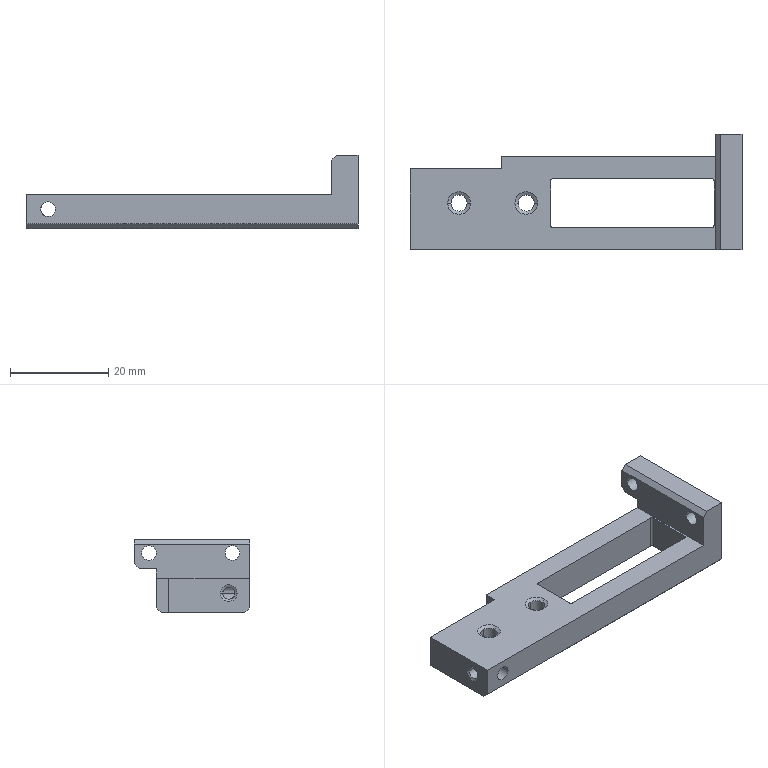Part | NX | 1 solid | 42 faces | box 67.7 x 23.5 x 15 mm | volume 6901 mm3 | plane 20 | cylinder 16 | cone 6 | commonest cylinder face diameters 3 x6 1 x4 3.3 x4 2.5 x2
STEP:
#1=CARTESIAN_POINT('',(-15.15,126.,-3.5));
#2=VERTEX_POINT('',#1);
#3=CARTESIAN_POINT('',(-33.85,126.,-3.5));
#4=VERTEX_POINT('',#3);
#5=CARTESIAN_POINT('',(0.,126.,-3.5));
#6=DIRECTION('',(-1.,0.,0.));
#7=VECTOR('',#6,1000.);
#8=LINE('',#5,#7);
#9=EDGE_CURVE('',#2,#4,#8,.T.);
#10=ORIENTED_EDGE('',*,*,#9,.T.);
#11=CARTESIAN_POINT('',(-33.85,126.,3.5));
#12=VERTEX_POINT('',#11);
#13=CARTESIAN_POINT('',(-33.85,126.,0.));
#14=DIRECTION('',(0.,0.,-1.));
#15=VECTOR('',#14,1000.);
#16=LINE('',#13,#15);
#17=EDGE_CURVE('',#12,#4,#16,.T.);
#18=ORIENTED_EDGE('',*,*,#17,.F.);
#19=CARTESIAN_POINT('',(-15.15,126.,3.5));
#20=VERTEX_POINT('',#19);
#21=CARTESIAN_POINT('',(0.,126.,3.5));
#22=DIRECTION('',(-1.,0.,0.));
#23=VECTOR('',#22,1000.);
#24=LINE('',#21,#23);
#25=EDGE_CURVE('',#20,#12,#24,.T.);
#26=ORIENTED_EDGE('',*,*,#25,.F.);
#27=CARTESIAN_POINT('',(-15.15,126.,-3.5));
#28=DIRECTION('',(0.,0.,1.));
#29=VECTOR('',#28,1000.);
#30=LINE('',#27,#29);
#31=EDGE_CURVE('',#2,#20,#30,.T.);
#32=ORIENTED_EDGE('',*,*,#31,.F.);
#33=EDGE_LOOP('',(#10,#18,#26,#32));
#34=FACE_BOUND('',#33,.T.);
#35=CARTESIAN_POINT('',(-30.85,126.,0.5));
#36=VERTEX_POINT('',#35);
#37=CARTESIAN_POINT('',(-27.85,126.,0.5));
#38=VERTEX_POINT('',#37);
#39=CARTESIAN_POINT('',(-29.35,126.,0.5));
#40=DIRECTION('',(0.,1.,0.));
#41=DIRECTION('',(-1.,0.,0.));
#42=AXIS2_PLACEMENT_3D('',#39,#40,#41);
#43=CIRCLE('',#42,1.5);
#44=EDGE_CURVE('',#36,#38,#43,.T.);
#45=ORIENTED_EDGE('',*,*,#44,.F.);
#46=CARTESIAN_POINT('',(-29.35,126.,0.5));
#47=DIRECTION('',(0.,1.,0.));
#48=DIRECTION('',(-1.,0.,0.));
#49=AXIS2_PLACEMENT_3D('',#46,#47,#48);
#50=CIRCLE('',#49,1.5);
#51=EDGE_CURVE('',#38,#36,#50,.T.);
#52=ORIENTED_EDGE('',*,*,#51,.F.);
#53=EDGE_LOOP('',(#45,#52));
#54=FACE_BOUND('',#53,.T.);
#55=CARTESIAN_POINT('',(-15.15,126.,3.5));
#56=DIRECTION('',(0.,1.,0.));
#57=DIRECTION('',(1.,0.,0.));
#58=AXIS2_PLACEMENT_3D('',#55,#56,#57);
#59=PLANE('',#58);
#60=ADVANCED_FACE('',(#34,#54),#59,.T.);
#61=CARTESIAN_POINT('',(-15.15,127.5,-3.5));
#62=VERTEX_POINT('',#61);
#63=CARTESIAN_POINT('',(-15.15,0.,-3.5));
#64=DIRECTION('',(0.,-1.,0.));
#65=VECTOR('',#64,1000.);
#66=LINE('',#63,#65);
#67=EDGE_CURVE('',#62,#2,#66,.T.);
#68=ORIENTED_EDGE('',*,*,#67,.T.);
#69=ORIENTED_EDGE('',*,*,#31,.T.);
#70=CARTESIAN_POINT('',(-15.15,128.5,3.5));
#71=VERTEX_POINT('',#70);
#72=CARTESIAN_POINT('',(-15.15,0.,3.5));
#73=DIRECTION('',(0.,-1.,0.));
#74=VECTOR('',#73,1000.);
#75=LINE('',#72,#74);
#76=EDGE_CURVE('',#71,#20,#75,.T.);
#77=ORIENTED_EDGE('',*,*,#76,.F.);
#78=CARTESIAN_POINT('',(-15.15,128.5,-2.5));
#79=VERTEX_POINT('',#78);
#80=CARTESIAN_POINT('',(-15.15,128.5,0.));
#81=DIRECTION('',(0.,0.,1.));
#82=VECTOR('',#81,1000.);
#83=LINE('',#80,#82);
#84=EDGE_CURVE('',#79,#71,#83,.T.);
#85=ORIENTED_EDGE('',*,*,#84,.F.);
#86=CARTESIAN_POINT('',(-15.15,127.5,-3.5));
#87=DIRECTION('',(0.,0.7071,0.7071));
#88=VECTOR('',#87,1000.);
#89=LINE('',#86,#88);
#90=EDGE_CURVE('',#62,#79,#89,.T.);
#91=ORIENTED_EDGE('',*,*,#90,.F.);
#92=EDGE_LOOP('',(#68,#69,#77,#85,#91));
#93=FACE_BOUND('',#92,.T.);
#94=CARTESIAN_POINT('',(-15.15,128.5,3.5));
#95=DIRECTION('',(-1.,0.,0.));
#96=DIRECTION('',(0.,0.,1.));
#97=AXIS2_PLACEMENT_3D('',#94,#95,#96);
#98=PLANE('',#97);
#99=ADVANCED_FACE('',(#93),#98,.T.);
#100=CARTESIAN_POINT('',(33.85,127.5,-3.5));
#101=VERTEX_POINT('',#100);
#102=CARTESIAN_POINT('',(0.,127.5,-3.5));
#103=DIRECTION('',(1.,0.,0.));
#104=VECTOR('',#103,1000.);
#105=LINE('',#102,#104);
#106=EDGE_CURVE('',#62,#101,#105,.T.);
#107=ORIENTED_EDGE('',*,*,#106,.F.);
#108=ORIENTED_EDGE('',*,*,#90,.T.);
#109=CARTESIAN_POINT('',(33.85,128.5,-2.5));
#110=VERTEX_POINT('',#109);
#111=CARTESIAN_POINT('',(0.,128.5,-2.5));
#112=DIRECTION('',(1.,0.,0.));
#113=VECTOR('',#112,1000.);
#114=LINE('',#111,#113);
#115=EDGE_CURVE('',#79,#110,#114,.T.);
#116=ORIENTED_EDGE('',*,*,#115,.T.);
#117=CARTESIAN_POINT('',(33.85,131.,0.));
#118=DIRECTION('',(0.,-0.7071,-0.7071));
#119=VECTOR('',#118,1000.);
#120=LINE('',#117,#119);
#121=EDGE_CURVE('',#110,#101,#120,.T.);
#122=ORIENTED_EDGE('',*,*,#121,.T.);
#123=EDGE_LOOP('',(#107,#108,#116,#122));
#124=FACE_BOUND('',#123,.T.);
#125=CARTESIAN_POINT('',(-15.15,127.5,-3.5));
#126=DIRECTION('',(0.,-0.7071,0.7071));
#127=DIRECTION('',(-1.,0.,0.));
#128=AXIS2_PLACEMENT_3D('',#125,#126,#127);
#129=PLANE('',#128);
#130=ADVANCED_FACE('',(#124),#129,.F.);
#131=ORIENTED_EDGE('',*,*,#76,.T.);
#132=ORIENTED_EDGE('',*,*,#25,.T.);
#133=CARTESIAN_POINT('',(-33.85,109.5,3.5));
#134=VERTEX_POINT('',#133);
#135=CARTESIAN_POINT('',(-33.85,0.,3.5));
#136=DIRECTION('',(0.,-1.,0.));
#137=VECTOR('',#136,1000.);
#138=LINE('',#135,#137);
#139=EDGE_CURVE('',#12,#134,#138,.T.);
#140=ORIENTED_EDGE('',*,*,#139,.T.);
#141=CARTESIAN_POINT('',(28.5,109.5,3.5));
#142=VERTEX_POINT('',#141);
#143=CARTESIAN_POINT('',(0.,109.5,3.5));
#144=DIRECTION('',(-1.,0.,0.));
#145=VECTOR('',#144,1000.);
#146=LINE('',#143,#145);
#147=EDGE_CURVE('',#142,#134,#146,.T.);
#148=ORIENTED_EDGE('',*,*,#147,.F.);
#149=CARTESIAN_POINT('',(28.5,128.5,3.5));
#150=VERTEX_POINT('',#149);
#151=CARTESIAN_POINT('',(28.5,0.,3.5));
#152=DIRECTION('',(0.,1.,0.));
#153=VECTOR('',#152,1000.);
#154=LINE('',#151,#153);
#155=EDGE_CURVE('',#142,#150,#154,.T.);
#156=ORIENTED_EDGE('',*,*,#155,.T.);
#157=CARTESIAN_POINT('',(0.,128.5,3.5));
#158=DIRECTION('',(1.,0.,0.));
#159=VECTOR('',#158,1000.);
#160=LINE('',#157,#159);
#161=EDGE_CURVE('',#71,#150,#160,.T.);
#162=ORIENTED_EDGE('',*,*,#161,.F.);
#163=EDGE_LOOP('',(#131,#132,#140,#148,#156,#162));
#164=FACE_BOUND('',#163,.T.);
#165=CARTESIAN_POINT('',(-4.65,124.,3.5));
#166=VERTEX_POINT('',#165);
#167=CARTESIAN_POINT('',(27.65,124.,3.5));
#168=VERTEX_POINT('',#167);
#169=CARTESIAN_POINT('',(0.,124.,3.5));
#170=DIRECTION('',(1.,0.,0.));
#171=VECTOR('',#170,1000.);
#172=LINE('',#169,#171);
#173=EDGE_CURVE('',#166,#168,#172,.T.);
#174=ORIENTED_EDGE('',*,*,#173,.T.);
#175=CARTESIAN_POINT('',(28.15,123.5,3.5));
#176=VERTEX_POINT('',#175);
#177=CARTESIAN_POINT('',(27.65,123.5,3.5));
#178=DIRECTION('',(0.,0.,-1.));
#179=DIRECTION('',(0.,-1.,0.));
#180=AXIS2_PLACEMENT_3D('',#177,#178,#179);
#181=CIRCLE('',#180,0.5);
#182=EDGE_CURVE('',#168,#176,#181,.T.);
#183=ORIENTED_EDGE('',*,*,#182,.T.);
#184=CARTESIAN_POINT('',(28.15,114.5,3.5));
#185=VERTEX_POINT('',#184);
#186=CARTESIAN_POINT('',(28.15,0.,3.5));
#187=DIRECTION('',(0.,-1.,0.));
#188=VECTOR('',#187,1000.);
#189=LINE('',#186,#188);
#190=EDGE_CURVE('',#176,#185,#189,.T.);
#191=ORIENTED_EDGE('',*,*,#190,.T.);
#192=CARTESIAN_POINT('',(27.65,114.,3.5));
#193=VERTEX_POINT('',#192);
#194=CARTESIAN_POINT('',(27.65,114.5,3.5));
#195=DIRECTION('',(0.,0.,-1.));
#196=DIRECTION('',(0.,-1.,0.));
#197=AXIS2_PLACEMENT_3D('',#194,#195,#196);
#198=CIRCLE('',#197,0.5);
#199=EDGE_CURVE('',#185,#193,#198,.T.);
#200=ORIENTED_EDGE('',*,*,#199,.T.);
#201=CARTESIAN_POINT('',(-4.65,114.,3.5));
#202=VERTEX_POINT('',#201);
#203=CARTESIAN_POINT('',(0.,114.,3.5));
#204=DIRECTION('',(-1.,0.,0.));
#205=VECTOR('',#204,1000.);
#206=LINE('',#203,#205);
#207=EDGE_CURVE('',#193,#202,#206,.T.);
#208=ORIENTED_EDGE('',*,*,#207,.T.);
#209=CARTESIAN_POINT('',(-5.15,114.5,3.5));
#210=VERTEX_POINT('',#209);
#211=CARTESIAN_POINT('',(-4.65,114.5,3.5));
#212=DIRECTION('',(0.,0.,-1.));
#213=DIRECTION('',(0.,-1.,0.));
#214=AXIS2_PLACEMENT_3D('',#211,#212,#213);
#215=CIRCLE('',#214,0.5);
#216=EDGE_CURVE('',#202,#210,#215,.T.);
#217=ORIENTED_EDGE('',*,*,#216,.T.);
#218=CARTESIAN_POINT('',(-5.15,123.5,3.5));
#219=VERTEX_POINT('',#218);
#220=CARTESIAN_POINT('',(-5.15,0.,3.5));
#221=DIRECTION('',(0.,1.,0.));
#222=VECTOR('',#221,1000.);
#223=LINE('',#220,#222);
#224=EDGE_CURVE('',#210,#219,#223,.T.);
#225=ORIENTED_EDGE('',*,*,#224,.T.);
#226=CARTESIAN_POINT('',(-4.65,123.5,3.5));
#227=DIRECTION('',(0.,0.,-1.));
#228=DIRECTION('',(0.,-1.,0.));
#229=AXIS2_PLACEMENT_3D('',#226,#227,#228);
#230=CIRCLE('',#229,0.5);
#231=EDGE_CURVE('',#219,#166,#230,.T.);
#232=ORIENTED_EDGE('',*,*,#231,.T.);
#233=EDGE_LOOP('',(#174,#183,#191,#200,#208,#217,#225,#232));
#234=FACE_BOUND('',#233,.T.);
#235=CARTESIAN_POINT('',(-21.535,119.,3.5));
#236=VERTEX_POINT('',#235);
#237=CARTESIAN_POINT('',(-26.165,119.,3.5));
#238=VERTEX_POINT('',#237);
#239=CARTESIAN_POINT('',(-23.85,119.,3.5));
#240=DIRECTION('',(0.,0.,1.));
#241=DIRECTION('',(1.,0.,0.));
#242=AXIS2_PLACEMENT_3D('',#239,#240,#241);
#243=CIRCLE('',#242,2.315);
#244=EDGE_CURVE('',#236,#238,#243,.T.);
#245=ORIENTED_EDGE('',*,*,#244,.F.);
#246=CARTESIAN_POINT('',(-23.85,119.,3.5));
#247=DIRECTION('',(0.,0.,1.));
#248=DIRECTION('',(1.,0.,0.));
#249=AXIS2_PLACEMENT_3D('',#246,#247,#248);
#250=CIRCLE('',#249,2.315);
#251=EDGE_CURVE('',#238,#236,#250,.T.);
#252=ORIENTED_EDGE('',*,*,#251,.F.);
#253=EDGE_LOOP('',(#245,#252));
#254=FACE_BOUND('',#253,.T.);
#255=CARTESIAN_POINT('',(-12.465,119.,3.5));
#256=VERTEX_POINT('',#255);
#257=CARTESIAN_POINT('',(-7.835,119.,3.5));
#258=VERTEX_POINT('',#257);
#259=CARTESIAN_POINT('',(-10.15,119.,3.5));
#260=DIRECTION('',(0.,0.,1.));
#261=DIRECTION('',(1.,0.,0.));
#262=AXIS2_PLACEMENT_3D('',#259,#260,#261);
#263=CIRCLE('',#262,2.315);
#264=EDGE_CURVE('',#256,#258,#263,.T.);
#265=ORIENTED_EDGE('',*,*,#264,.F.);
#266=CARTESIAN_POINT('',(-10.15,119.,3.5));
#267=DIRECTION('',(0.,0.,1.));
#268=DIRECTION('',(1.,0.,0.));
#269=AXIS2_PLACEMENT_3D('',#266,#267,#268);
#270=CIRCLE('',#269,2.315);
#271=EDGE_CURVE('',#258,#256,#270,.T.);
#272=ORIENTED_EDGE('',*,*,#271,.F.);
#273=EDGE_LOOP('',(#265,#272));
#274=FACE_BOUND('',#273,.T.);
#275=CARTESIAN_POINT('',(0.,119.,3.5));
#276=DIRECTION('',(0.,0.,-1.));
#277=DIRECTION('',(0.,-1.,0.));
#278=AXIS2_PLACEMENT_3D('',#275,#276,#277);
#279=PLANE('',#278);
#280=ADVANCED_FACE('',(#164,#234,#254,#274),#279,.F.);
#281=CARTESIAN_POINT('',(29.5,109.5,11.5));
#282=VERTEX_POINT('',#281);
#283=CARTESIAN_POINT('',(29.5,133.,11.5));
#284=VERTEX_POINT('',#283);
#285=CARTESIAN_POINT('',(29.5,0.,11.5));
#286=DIRECTION('',(0.,1.,0.));
#287=VECTOR('',#286,1000.);
#288=LINE('',#285,#287);
#289=EDGE_CURVE('',#282,#284,#288,.T.);
#290=ORIENTED_EDGE('',*,*,#289,.F.);
#291=CARTESIAN_POINT('',(33.85,109.5,11.5));
#292=VERTEX_POINT('',#291);
#293=CARTESIAN_POINT('',(0.,109.5,11.5));
#294=DIRECTION('',(1.,0.,0.));
#295=VECTOR('',#294,1000.);
#296=LINE('',#293,#295);
#297=EDGE_CURVE('',#282,#292,#296,.T.);
#298=ORIENTED_EDGE('',*,*,#297,.T.);
#299=CARTESIAN_POINT('',(33.85,133.,11.5));
#300=VERTEX_POINT('',#299);
#301=CARTESIAN_POINT('',(33.85,0.,11.5));
#302=DIRECTION('',(0.,1.,0.));
#303=VECTOR('',#302,1000.);
#304=LINE('',#301,#303);
#305=EDGE_CURVE('',#292,#300,#304,.T.);
#306=ORIENTED_EDGE('',*,*,#305,.T.);
#307=CARTESIAN_POINT('',(0.,133.,11.5));
#308=DIRECTION('',(1.,0.,0.));
#309=VECTOR('',#308,1000.);
#310=LINE('',#307,#309);
#311=EDGE_CURVE('',#284,#300,#310,.T.);
#312=ORIENTED_EDGE('',*,*,#311,.F.);
#313=EDGE_LOOP('',(#290,#298,#306,#312));
#314=FACE_BOUND('',#313,.T.);
#315=CARTESIAN_POINT('',(0.,119.,11.5));
#316=DIRECTION('',(0.,0.,-1.));
#317=DIRECTION('',(0.,-1.,0.));
#318=AXIS2_PLACEMENT_3D('',#315,#316,#317);
#319=PLANE('',#318);
#320=ADVANCED_FACE('',(#314),#319,.F.);
#321=CARTESIAN_POINT('',(28.5,109.5,10.5));
#322=VERTEX_POINT('',#321);
#323=CARTESIAN_POINT('',(28.5,133.,10.5));
#324=VERTEX_POINT('',#323);
#325=CARTESIAN_POINT('',(28.5,0.,10.5));
#326=DIRECTION('',(0.,1.,0.));
#327=VECTOR('',#326,1000.);
#328=LINE('',#325,#327);
#329=EDGE_CURVE('',#322,#324,#328,.T.);
#330=ORIENTED_EDGE('',*,*,#329,.F.);
#331=CARTESIAN_POINT('',(18.,109.5,0.));
#332=DIRECTION('',(-0.7071,0.,-0.7071));
#333=VECTOR('',#332,1000.);
#334=LINE('',#331,#333);
#335=EDGE_CURVE('',#282,#322,#334,.T.);
#336=ORIENTED_EDGE('',*,*,#335,.F.);
#337=ORIENTED_EDGE('',*,*,#289,.T.);
#338=CARTESIAN_POINT('',(18.,133.,0.));
#339=DIRECTION('',(-0.7071,0.,-0.7071));
#340=VECTOR('',#339,1000.);
#341=LINE('',#338,#340);
#342=EDGE_CURVE('',#284,#324,#341,.T.);
#343=ORIENTED_EDGE('',*,*,#342,.T.);
#344=EDGE_LOOP('',(#330,#336,#337,#343));
#345=FACE_BOUND('',#344,.T.);
#346=CARTESIAN_POINT('',(28.5,129.5,10.5));
#347=DIRECTION('',(-0.7071,0.,0.7071));
#348=DIRECTION('',(0.,1.,0.));
#349=AXIS2_PLACEMENT_3D('',#346,#347,#348);
#350=PLANE('',#349);
#351=ADVANCED_FACE('',(#345),#350,.T.);
#352=CARTESIAN_POINT('',(-33.85,110.5,-3.5));
#353=VERTEX_POINT('',#352);
#354=CARTESIAN_POINT('',(33.85,110.5,-3.5));
#355=VERTEX_POINT('',#354);
#356=CARTESIAN_POINT('',(0.,110.5,-3.5));
#357=DIRECTION('',(1.,0.,0.));
#358=VECTOR('',#357,1000.);
#359=LINE('',#356,#358);
#360=EDGE_CURVE('',#353,#355,#359,.T.);
#361=ORIENTED_EDGE('',*,*,#360,.F.);
#362=CARTESIAN_POINT('',(-33.85,0.,-3.5));
#363=DIRECTION('',(0.,-1.,0.));
#364=VECTOR('',#363,1000.);
#365=LINE('',#362,#364);
#366=EDGE_CURVE('',#4,#353,#365,.T.);
#367=ORIENTED_EDGE('',*,*,#366,.F.);
#368=ORIENTED_EDGE('',*,*,#9,.F.);
#369=ORIENTED_EDGE('',*,*,#67,.F.);
#370=ORIENTED_EDGE('',*,*,#106,.T.);
#371=CARTESIAN_POINT('',(33.85,0.,-3.5));
#372=DIRECTION('',(0.,-1.,0.));
#373=VECTOR('',#372,1000.);
#374=LINE('',#371,#373);
#375=EDGE_CURVE('',#101,#355,#374,.T.);
#376=ORIENTED_EDGE('',*,*,#375,.T.);
#377=EDGE_LOOP('',(#361,#367,#368,#369,#370,#376));
#378=FACE_BOUND('',#377,.T.);
#379=CARTESIAN_POINT('',(-4.65,124.,-3.5));
#380=VERTEX_POINT('',#379);
#381=CARTESIAN_POINT('',(27.65,124.,-3.5));
#382=VERTEX_POINT('',#381);
#383=CARTESIAN_POINT('',(0.,124.,-3.5));
#384=DIRECTION('',(1.,0.,0.));
#385=VECTOR('',#384,1000.);
#386=LINE('',#383,#385);
#387=EDGE_CURVE('',#380,#382,#386,.T.);
#388=ORIENTED_EDGE('',*,*,#387,.F.);
#389=CARTESIAN_POINT('',(-5.15,123.5,-3.5));
#390=VERTEX_POINT('',#389);
#391=CARTESIAN_POINT('',(-4.65,123.5,-3.5));
#392=DIRECTION('',(0.,0.,-1.));
#393=DIRECTION('',(0.,-1.,0.));
#394=AXIS2_PLACEMENT_3D('',#391,#392,#393);
#395=CIRCLE('',#394,0.5);
#396=EDGE_CURVE('',#390,#380,#395,.T.);
#397=ORIENTED_EDGE('',*,*,#396,.F.);
#398=CARTESIAN_POINT('',(-5.15,114.5,-3.5));
#399=VERTEX_POINT('',#398);
#400=CARTESIAN_POINT('',(-5.15,0.,-3.5));
#401=DIRECTION('',(0.,1.,0.));
#402=VECTOR('',#401,1000.);
#403=LINE('',#400,#402);
#404=EDGE_CURVE('',#399,#390,#403,.T.);
#405=ORIENTED_EDGE('',*,*,#404,.F.);
#406=CARTESIAN_POINT('',(-4.65,114.,-3.5));
#407=VERTEX_POINT('',#406);
#408=CARTESIAN_POINT('',(-4.65,114.5,-3.5));
#409=DIRECTION('',(0.,0.,-1.));
#410=DIRECTION('',(0.,-1.,0.));
#411=AXIS2_PLACEMENT_3D('',#408,#409,#410);
#412=CIRCLE('',#411,0.5);
#413=EDGE_CURVE('',#407,#399,#412,.T.);
#414=ORIENTED_EDGE('',*,*,#413,.F.);
#415=CARTESIAN_POINT('',(27.65,114.,-3.5));
#416=VERTEX_POINT('',#415);
#417=CARTESIAN_POINT('',(0.,114.,-3.5));
#418=DIRECTION('',(-1.,0.,0.));
#419=VECTOR('',#418,1000.);
#420=LINE('',#417,#419);
#421=EDGE_CURVE('',#416,#407,#420,.T.);
#422=ORIENTED_EDGE('',*,*,#421,.F.);
#423=CARTESIAN_POINT('',(28.15,114.5,-3.5));
#424=VERTEX_POINT('',#423);
#425=CARTESIAN_POINT('',(27.65,114.5,-3.5));
#426=DIRECTION('',(0.,0.,-1.));
#427=DIRECTION('',(0.,-1.,0.));
#428=AXIS2_PLACEMENT_3D('',#425,#426,#427);
#429=CIRCLE('',#428,0.5);
#430=EDGE_CURVE('',#424,#416,#429,.T.);
#431=ORIENTED_EDGE('',*,*,#430,.F.);
#432=CARTESIAN_POINT('',(28.15,123.5,-3.5));
#433=VERTEX_POINT('',#432);
#434=CARTESIAN_POINT('',(28.15,0.,-3.5));
#435=DIRECTION('',(0.,-1.,0.));
#436=VECTOR('',#435,1000.);
#437=LINE('',#434,#436);
#438=EDGE_CURVE('',#433,#424,#437,.T.);
#439=ORIENTED_EDGE('',*,*,#438,.F.);
#440=CARTESIAN_POINT('',(27.65,123.5,-3.5));
#441=DIRECTION('',(0.,0.,-1.));
#442=DIRECTION('',(0.,-1.,0.));
#443=AXIS2_PLACEMENT_3D('',#440,#441,#442);
#444=CIRCLE('',#443,0.5);
#445=EDGE_CURVE('',#382,#433,#444,.T.);
#446=ORIENTED_EDGE('',*,*,#445,.F.);
#447=EDGE_LOOP('',(#388,#397,#405,#414,#422,#431,#439,#446));
#448=FACE_BOUND('',#447,.T.);
#449=CARTESIAN_POINT('',(-10.15,117.35,-3.5));
#450=VERTEX_POINT('',#449);
#451=CARTESIAN_POINT('',(-10.15,120.65,-3.5));
#452=VERTEX_POINT('',#451);
#453=CARTESIAN_POINT('',(-10.15,119.,-3.5));
#454=DIRECTION('',(0.,0.,1.));
#455=DIRECTION('',(0.,1.,0.));
#456=AXIS2_PLACEMENT_3D('',#453,#454,#455);
#457=CIRCLE('',#456,1.65);
#458=EDGE_CURVE('',#450,#452,#457,.T.);
#459=ORIENTED_EDGE('',*,*,#458,.T.);
#460=CARTESIAN_POINT('',(-10.15,119.,-3.5));
#461=DIRECTION('',(0.,0.,1.));
#462=DIRECTION('',(0.,1.,0.));
#463=AXIS2_PLACEMENT_3D('',#460,#461,#462);
#464=CIRCLE('',#463,1.65);
#465=EDGE_CURVE('',#452,#450,#464,.T.);
#466=ORIENTED_EDGE('',*,*,#465,.T.);
#467=EDGE_LOOP('',(#459,#466));
#468=FACE_BOUND('',#467,.T.);
#469=CARTESIAN_POINT('',(-23.85,117.35,-3.5));
#470=VERTEX_POINT('',#469);
#471=CARTESIAN_POINT('',(-23.85,120.65,-3.5));
#472=VERTEX_POINT('',#471);
#473=CARTESIAN_POINT('',(-23.85,119.,-3.5));
#474=DIRECTION('',(0.,0.,1.));
#475=DIRECTION('',(0.,1.,0.));
#476=AXIS2_PLACEMENT_3D('',#473,#474,#475);
#477=CIRCLE('',#476,1.65);
#478=EDGE_CURVE('',#470,#472,#477,.T.);
#479=ORIENTED_EDGE('',*,*,#478,.T.);
#480=CARTESIAN_POINT('',(-23.85,119.,-3.5));
#481=DIRECTION('',(0.,0.,1.));
#482=DIRECTION('',(0.,1.,0.));
#483=AXIS2_PLACEMENT_3D('',#480,#481,#482);
#484=CIRCLE('',#483,1.65);
#485=EDGE_CURVE('',#472,#470,#484,.T.);
#486=ORIENTED_EDGE('',*,*,#485,.T.);
#487=EDGE_LOOP('',(#479,#486));
#488=FACE_BOUND('',#487,.T.);
#489=CARTESIAN_POINT('',(0.,119.,-3.5));
#490=DIRECTION('',(0.,0.,-1.));
#491=DIRECTION('',(0.,-1.,0.));
#492=AXIS2_PLACEMENT_3D('',#489,#490,#491);
#493=PLANE('',#492);
#494=ADVANCED_FACE('',(#378,#448,#468,#488),#493,.T.);
#495=CARTESIAN_POINT('',(28.5,128.5,5.5));
#496=VERTEX_POINT('',#495);
#497=CARTESIAN_POINT('',(33.85,128.5,5.5));
#498=VERTEX_POINT('',#497);
#499=CARTESIAN_POINT('',(0.,128.5,5.5));
#500=DIRECTION('',(1.,0.,0.));
#501=VECTOR('',#500,1000.);
#502=LINE('',#499,#501);
#503=EDGE_CURVE('',#496,#498,#502,.T.);
#504=ORIENTED_EDGE('',*,*,#503,.T.);
#505=CARTESIAN_POINT('',(33.85,128.5,0.));
#506=DIRECTION('',(0.,0.,-1.));
#507=VECTOR('',#506,1000.);
#508=LINE('',#505,#507);
#509=EDGE_CURVE('',#498,#110,#508,.T.);
#510=ORIENTED_EDGE('',*,*,#509,.T.);
#511=ORIENTED_EDGE('',*,*,#115,.F.);
#512=ORIENTED_EDGE('',*,*,#84,.T.);
#513=ORIENTED_EDGE('',*,*,#161,.T.);
#514=CARTESIAN_POINT('',(28.5,128.5,0.));
#515=DIRECTION('',(0.,0.,1.));
#516=VECTOR('',#515,1000.);
#517=LINE('',#514,#516);
#518=EDGE_CURVE('',#150,#496,#517,.T.);
#519=ORIENTED_EDGE('',*,*,#518,.T.);
#520=EDGE_LOOP('',(#504,#510,#511,#512,#513,#519));
#521=FACE_BOUND('',#520,.T.);
#522=CARTESIAN_POINT('',(-33.85,128.5,-3.5));
#523=DIRECTION('',(0.,-1.,0.));
#524=DIRECTION('',(0.,0.,-1.));
#525=AXIS2_PLACEMENT_3D('',#522,#523,#524);
#526=PLANE('',#525);
#527=ADVANCED_FACE('',(#521),#526,.F.);
#528=CARTESIAN_POINT('',(33.85,132.,5.5));
#529=VERTEX_POINT('',#528);
#530=CARTESIAN_POINT('',(28.5,132.,5.5));
#531=VERTEX_POINT('',#530);
#532=CARTESIAN_POINT('',(0.,132.,5.5));
#533=DIRECTION('',(-1.,0.,0.));
#534=VECTOR('',#533,1000.);
#535=LINE('',#532,#534);
#536=EDGE_CURVE('',#529,#531,#535,.T.);
#537=ORIENTED_EDGE('',*,*,#536,.F.);
#538=CARTESIAN_POINT('',(33.85,0.,5.5));
#539=DIRECTION('',(0.,1.,0.));
#540=VECTOR('',#539,1000.);
#541=LINE('',#538,#540);
#542=EDGE_CURVE('',#498,#529,#541,.T.);
#543=ORIENTED_EDGE('',*,*,#542,.F.);
#544=ORIENTED_EDGE('',*,*,#503,.F.);
#545=CARTESIAN_POINT('',(28.5,0.,5.5));
#546=DIRECTION('',(0.,-1.,0.));
#547=VECTOR('',#546,1000.);
#548=LINE('',#545,#547);
#549=EDGE_CURVE('',#531,#496,#548,.T.);
#550=ORIENTED_EDGE('',*,*,#549,.F.);
#551=EDGE_LOOP('',(#537,#543,#544,#550));
#552=FACE_BOUND('',#551,.T.);
#553=CARTESIAN_POINT('',(33.85,128.5,5.5));
#554=DIRECTION('',(0.,0.,-1.));
#555=DIRECTION('',(0.,-1.,0.));
#556=AXIS2_PLACEMENT_3D('',#553,#554,#555);
#557=PLANE('',#556);
#558=ADVANCED_FACE('',(#552),#557,.T.);
#559=ORIENTED_EDGE('',*,*,#311,.T.);
#560=CARTESIAN_POINT('',(33.85,133.,6.5));
#561=VERTEX_POINT('',#560);
#562=CARTESIAN_POINT('',(33.85,133.,0.));
#563=DIRECTION('',(0.,0.,1.));
#564=VECTOR('',#563,1000.);
#565=LINE('',#562,#564);
#566=EDGE_CURVE('',#561,#300,#565,.T.);
#567=ORIENTED_EDGE('',*,*,#566,.F.);
#568=CARTESIAN_POINT('',(28.5,133.,6.5));
#569=VERTEX_POINT('',#568);
#570=CARTESIAN_POINT('',(0.,133.,6.5));
#571=DIRECTION('',(1.,0.,0.));
#572=VECTOR('',#571,1000.);
#573=LINE('',#570,#572);
#574=EDGE_CURVE('',#569,#561,#573,.T.);
#575=ORIENTED_EDGE('',*,*,#574,.F.);
#576=CARTESIAN_POINT('',(28.5,133.,0.));
#577=DIRECTION('',(0.,0.,-1.));
#578=VECTOR('',#577,1000.);
#579=LINE('',#576,#578);
#580=EDGE_CURVE('',#324,#569,#579,.T.);
#581=ORIENTED_EDGE('',*,*,#580,.F.);
#582=ORIENTED_EDGE('',*,*,#342,.F.);
#583=EDGE_LOOP('',(#559,#567,#575,#581,#582));
#584=FACE_BOUND('',#583,.T.);
#585=CARTESIAN_POINT('',(0.,133.,-3.5));
#586=DIRECTION('',(0.,1.,0.));
#587=DIRECTION('',(1.,0.,0.));
#588=AXIS2_PLACEMENT_3D('',#585,#586,#587);
#589=PLANE('',#588);
#590=ADVANCED_FACE('',(#584),#589,.T.);
#591=CARTESIAN_POINT('',(-30.85,115.,0.5));
#592=VERTEX_POINT('',#591);
#593=CARTESIAN_POINT('',(-30.85,112.5,0.5));
#594=VERTEX_POINT('',#593);
#595=CARTESIAN_POINT('',(-30.85,115.,0.5));
#596=CARTESIAN_POINT('',(-30.85,115.,0.6668));
#597=CARTESIAN_POINT('',(-30.788,114.924,0.9606));
#598=CARTESIAN_POINT('',(-30.695,114.813,1.179));
#599=CARTESIAN_POINT('',(-30.553,114.621,1.399));
#600=CARTESIAN_POINT('',(-30.53,114.592,1.427));
#601=CARTESIAN_POINT('',(-30.39,114.384,1.589));
#602=CARTESIAN_POINT('',(-30.284,114.198,1.674));
#603=CARTESIAN_POINT('',(-30.109,113.75,1.801));
#604=CARTESIAN_POINT('',(-30.284,113.301,1.674));
#605=CARTESIAN_POINT('',(-30.39,113.116,1.59));
#606=CARTESIAN_POINT('',(-30.531,112.907,1.426));
#607=CARTESIAN_POINT('',(-30.552,112.88,1.399));
#608=CARTESIAN_POINT('',(-30.695,112.687,1.179));
#609=CARTESIAN_POINT('',(-30.788,112.576,0.9603));
#610=CARTESIAN_POINT('',(-30.85,112.5,0.6667));
#611=CARTESIAN_POINT('',(-30.85,112.5,0.5));
#612=B_SPLINE_CURVE_WITH_KNOTS('',3,(#595,#596,#597,#598,#599,#600,#601,#602,#603,#604,#605,#606,#607,#608,#609,#610,#611),.UNSPECIFIED.,.F.,.F.,(4,1,1,1,1,1,1,1,1,1,1,1,1,1,4),(0.,0.125,0.1875,0.25,0.2812,0.3125,0.375,0.5,0.625,0.6875,0.7188,0.75,0.8125,0.875,1.),.UNSPECIFIED.);
#613=EDGE_CURVE('',#592,#594,#612,.T.);
#614=ORIENTED_EDGE('',*,*,#613,.T.);
#615=CARTESIAN_POINT('',(-33.59,112.5,0.5));
#616=VERTEX_POINT('',#615);
#617=CARTESIAN_POINT('',(-32.015,112.5,0.5));
#618=DIRECTION('',(-1.,0.,0.));
#619=VECTOR('',#618,1000.);
#620=LINE('',#617,#619);
#621=EDGE_CURVE('',#616,#594,#620,.F.);
#622=ORIENTED_EDGE('',*,*,#621,.F.);
#623=CARTESIAN_POINT('',(-33.59,115.,0.5));
#624=VERTEX_POINT('',#623);
#625=CARTESIAN_POINT('',(-33.59,113.75,0.5));
#626=DIRECTION('',(-1.,0.,0.));
#627=DIRECTION('',(0.,1.,0.));
#628=AXIS2_PLACEMENT_3D('',#625,#626,#627);
#629=CIRCLE('',#628,1.25);
#630=EDGE_CURVE('',#616,#624,#629,.T.);
#631=ORIENTED_EDGE('',*,*,#630,.T.);
#632=CARTESIAN_POINT('',(-32.015,115.,0.5));
#633=DIRECTION('',(-1.,0.,0.));
#634=VECTOR('',#633,1000.);
#635=LINE('',#632,#634);
#636=EDGE_CURVE('',#624,#592,#635,.F.);
#637=ORIENTED_EDGE('',*,*,#636,.T.);
#638=EDGE_LOOP('',(#614,#622,#631,#637));
#639=FACE_BOUND('',#638,.T.);
#640=CARTESIAN_POINT('',(-32.015,113.75,0.5));
#641=DIRECTION('',(-1.,0.,0.));
#642=DIRECTION('',(0.,-1.,0.));
#643=AXIS2_PLACEMENT_3D('',#640,#641,#642);
#644=CYLINDRICAL_SURFACE('',#643,1.25);
#645=ADVANCED_FACE('',(#639),#644,.F.);
#646=ORIENTED_EDGE('',*,*,#17,.T.);
#647=ORIENTED_EDGE('',*,*,#366,.T.);
#648=CARTESIAN_POINT('',(-33.85,109.5,-2.5));
#649=VERTEX_POINT('',#648);
#650=CARTESIAN_POINT('',(-33.85,107.,0.));
#651=DIRECTION('',(0.,-0.7071,0.7071));
#652=VECTOR('',#651,1000.);
#653=LINE('',#650,#652);
#654=EDGE_CURVE('',#353,#649,#653,.T.);
#655=ORIENTED_EDGE('',*,*,#654,.T.);
#656=CARTESIAN_POINT('',(-33.85,109.5,0.));
#657=DIRECTION('',(0.,0.,1.));
#658=VECTOR('',#657,1000.);
#659=LINE('',#656,#658);
#660=EDGE_CURVE('',#649,#134,#659,.T.);
#661=ORIENTED_EDGE('',*,*,#660,.T.);
#662=ORIENTED_EDGE('',*,*,#139,.F.);
#663=EDGE_LOOP('',(#646,#647,#655,#661,#662));
#664=FACE_BOUND('',#663,.T.);
#665=CARTESIAN_POINT('',(-33.85,115.45,0.5));
#666=VERTEX_POINT('',#665);
#667=CARTESIAN_POINT('',(-33.85,112.05,0.5));
#668=VERTEX_POINT('',#667);
#669=CARTESIAN_POINT('',(-33.85,113.75,0.5));
#670=DIRECTION('',(-1.,0.,0.));
#671=DIRECTION('',(0.,1.,0.));
#672=AXIS2_PLACEMENT_3D('',#669,#670,#671);
#673=CIRCLE('',#672,1.7);
#674=EDGE_CURVE('',#666,#668,#673,.T.);
#675=ORIENTED_EDGE('',*,*,#674,.F.);
#676=CARTESIAN_POINT('',(-33.85,113.75,0.5));
#677=DIRECTION('',(-1.,0.,0.));
#678=DIRECTION('',(0.,1.,0.));
#679=AXIS2_PLACEMENT_3D('',#676,#677,#678);
#680=CIRCLE('',#679,1.7);
#681=EDGE_CURVE('',#668,#666,#680,.T.);
#682=ORIENTED_EDGE('',*,*,#681,.F.);
#683=EDGE_LOOP('',(#675,#682));
#684=FACE_BOUND('',#683,.T.);
#685=CARTESIAN_POINT('',(-33.85,109.5,-3.5));
#686=DIRECTION('',(1.,0.,0.));
#687=DIRECTION('',(0.,1.,0.));
#688=AXIS2_PLACEMENT_3D('',#685,#686,#687);
#689=PLANE('',#688);
#690=ADVANCED_FACE('',(#664,#684),#689,.F.);
#691=CARTESIAN_POINT('',(-33.59,113.75,0.5));
#692=DIRECTION('',(-1.,0.,0.));
#693=DIRECTION('',(0.,1.,0.));
#694=AXIS2_PLACEMENT_3D('',#691,#692,#693);
#695=CIRCLE('',#694,1.25);
#696=EDGE_CURVE('',#624,#616,#695,.T.);
#697=ORIENTED_EDGE('',*,*,#696,.F.);
#698=CARTESIAN_POINT('',(-33.59,115.,0.5));
#699=DIRECTION('',(-0.5,0.866,0.));
#700=VECTOR('',#699,1000.);
#701=LINE('',#698,#700);
#702=EDGE_CURVE('',#624,#666,#701,.T.);
#703=ORIENTED_EDGE('',*,*,#702,.T.);
#704=ORIENTED_EDGE('',*,*,#674,.T.);
#705=CARTESIAN_POINT('',(-33.59,112.5,0.5));
#706=DIRECTION('',(-0.5,-0.866,0.));
#707=VECTOR('',#706,1000.);
#708=LINE('',#705,#707);
#709=EDGE_CURVE('',#616,#668,#708,.T.);
#710=ORIENTED_EDGE('',*,*,#709,.F.);
#711=EDGE_LOOP('',(#697,#703,#704,#710));
#712=FACE_BOUND('',#711,.T.);
#713=CARTESIAN_POINT('',(-33.59,113.75,0.5));
#714=DIRECTION('',(-1.,0.,0.));
#715=DIRECTION('',(0.,1.,0.));
#716=AXIS2_PLACEMENT_3D('',#713,#714,#715);
#717=CONICAL_SURFACE('',#716,1.25,1.047);
#718=ADVANCED_FACE('',(#712),#717,.F.);
#719=ORIENTED_EDGE('',*,*,#518,.F.);
#720=ORIENTED_EDGE('',*,*,#155,.F.);
#721=CARTESIAN_POINT('',(28.5,109.5,0.));
#722=DIRECTION('',(0.,0.,1.));
#723=VECTOR('',#722,1000.);
#724=LINE('',#721,#723);
#725=EDGE_CURVE('',#142,#322,#724,.T.);
#726=ORIENTED_EDGE('',*,*,#725,.T.);
#727=ORIENTED_EDGE('',*,*,#329,.T.);
#728=ORIENTED_EDGE('',*,*,#580,.T.);
#729=CARTESIAN_POINT('',(28.5,126.5,0.));
#730=DIRECTION('',(0.,-0.7071,-0.7071));
#731=VECTOR('',#730,1000.);
#732=LINE('',#729,#731);
#733=EDGE_CURVE('',#569,#531,#732,.T.);
#734=ORIENTED_EDGE('',*,*,#733,.T.);
#735=ORIENTED_EDGE('',*,*,#549,.T.);
#736=EDGE_LOOP('',(#719,#720,#726,#727,#728,#734,#735));
#737=FACE_BOUND('',#736,.T.);
#738=CARTESIAN_POINT('',(28.5,128.5,8.68));
#739=VERTEX_POINT('',#738);
#740=CARTESIAN_POINT('',(28.5,131.5,8.68));
#741=VERTEX_POINT('',#740);
#742=CARTESIAN_POINT('',(28.5,130.,8.68));
#743=DIRECTION('',(-1.,0.,0.));
#744=DIRECTION('',(0.,-1.,0.));
#745=AXIS2_PLACEMENT_3D('',#742,#743,#744);
#746=CIRCLE('',#745,1.5);
#747=EDGE_CURVE('',#739,#741,#746,.T.);
#748=ORIENTED_EDGE('',*,*,#747,.F.);
#749=CARTESIAN_POINT('',(28.5,130.,8.68));
#750=DIRECTION('',(-1.,0.,0.));
#751=DIRECTION('',(0.,-1.,0.));
#752=AXIS2_PLACEMENT_3D('',#749,#750,#751);
#753=CIRCLE('',#752,1.5);
#754=EDGE_CURVE('',#741,#739,#753,.T.);
#755=ORIENTED_EDGE('',*,*,#754,.F.);
#756=EDGE_LOOP('',(#748,#755));
#757=FACE_BOUND('',#756,.T.);
#758=CARTESIAN_POINT('',(28.5,111.5,8.68));
#759=VERTEX_POINT('',#758);
#760=CARTESIAN_POINT('',(28.5,114.5,8.68));
#761=VERTEX_POINT('',#760);
#762=CARTESIAN_POINT('',(28.5,113.,8.68));
#763=DIRECTION('',(-1.,0.,0.));
#764=DIRECTION('',(0.,-1.,0.));
#765=AXIS2_PLACEMENT_3D('',#762,#763,#764);
#766=CIRCLE('',#765,1.5);
#767=EDGE_CURVE('',#759,#761,#766,.T.);
#768=ORIENTED_EDGE('',*,*,#767,.F.);
#769=CARTESIAN_POINT('',(28.5,113.,8.68));
#770=DIRECTION('',(-1.,0.,0.));
#771=DIRECTION('',(0.,-1.,0.));
#772=AXIS2_PLACEMENT_3D('',#769,#770,#771);
#773=CIRCLE('',#772,1.5);
#774=EDGE_CURVE('',#761,#759,#773,.T.);
#775=ORIENTED_EDGE('',*,*,#774,.F.);
#776=EDGE_LOOP('',(#768,#775));
#777=FACE_BOUND('',#776,.T.);
#778=CARTESIAN_POINT('',(28.5,109.5,3.5));
#779=DIRECTION('',(1.,0.,0.));
#780=DIRECTION('',(0.,1.,0.));
#781=AXIS2_PLACEMENT_3D('',#778,#779,#780);
#782=PLANE('',#781);
#783=ADVANCED_FACE('',(#737,#757,#777),#782,.F.);
#784=CARTESIAN_POINT('',(33.85,109.5,-2.5));
#785=VERTEX_POINT('',#784);
#786=CARTESIAN_POINT('',(0.,109.5,-2.5));
#787=DIRECTION('',(1.,0.,0.));
#788=VECTOR('',#787,1000.);
#789=LINE('',#786,#788);
#790=EDGE_CURVE('',#649,#785,#789,.T.);
#791=ORIENTED_EDGE('',*,*,#790,.T.);
#792=CARTESIAN_POINT('',(33.85,109.5,0.));
#793=DIRECTION('',(0.,0.,1.));
#794=VECTOR('',#793,1000.);
#795=LINE('',#792,#794);
#796=EDGE_CURVE('',#785,#292,#795,.T.);
#797=ORIENTED_EDGE('',*,*,#796,.T.);
#798=ORIENTED_EDGE('',*,*,#297,.F.);
#799=ORIENTED_EDGE('',*,*,#335,.T.);
#800=ORIENTED_EDGE('',*,*,#725,.F.);
#801=ORIENTED_EDGE('',*,*,#147,.T.);
#802=ORIENTED_EDGE('',*,*,#660,.F.);
#803=EDGE_LOOP('',(#791,#797,#798,#799,#800,#801,#802));
#804=FACE_BOUND('',#803,.T.);
#805=CARTESIAN_POINT('',(-30.85,109.5,0.5));
#806=VERTEX_POINT('',#805);
#807=CARTESIAN_POINT('',(-27.85,109.5,0.5));
#808=VERTEX_POINT('',#807);
#809=CARTESIAN_POINT('',(-29.35,109.5,0.5));
#810=DIRECTION('',(0.,1.,0.));
#811=DIRECTION('',(-1.,0.,0.));
#812=AXIS2_PLACEMENT_3D('',#809,#810,#811);
#813=CIRCLE('',#812,1.5);
#814=EDGE_CURVE('',#806,#808,#813,.T.);
#815=ORIENTED_EDGE('',*,*,#814,.T.);
#816=CARTESIAN_POINT('',(-29.35,109.5,0.5));
#817=DIRECTION('',(0.,1.,0.));
#818=DIRECTION('',(-1.,0.,0.));
#819=AXIS2_PLACEMENT_3D('',#816,#817,#818);
#820=CIRCLE('',#819,1.5);
#821=EDGE_CURVE('',#808,#806,#820,.T.);
#822=ORIENTED_EDGE('',*,*,#821,.T.);
#823=EDGE_LOOP('',(#815,#822));
#824=FACE_BOUND('',#823,.T.);
#825=CARTESIAN_POINT('',(33.85,109.5,-3.5));
#826=DIRECTION('',(0.,1.,0.));
#827=DIRECTION('',(1.,0.,0.));
#828=AXIS2_PLACEMENT_3D('',#825,#826,#827);
#829=PLANE('',#828);
#830=ADVANCED_FACE('',(#804,#824),#829,.F.);
#831=ORIENTED_EDGE('',*,*,#375,.F.);
#832=ORIENTED_EDGE('',*,*,#121,.F.);
#833=ORIENTED_EDGE('',*,*,#509,.F.);
#834=ORIENTED_EDGE('',*,*,#542,.T.);
#835=CARTESIAN_POINT('',(33.85,126.5,0.));
#836=DIRECTION('',(0.,0.7071,0.7071));
#837=VECTOR('',#836,1000.);
#838=LINE('',#835,#837);
#839=EDGE_CURVE('',#529,#561,#838,.T.);
#840=ORIENTED_EDGE('',*,*,#839,.T.);
#841=ORIENTED_EDGE('',*,*,#566,.T.);
#842=ORIENTED_EDGE('',*,*,#305,.F.);
#843=ORIENTED_EDGE('',*,*,#796,.F.);
#844=CARTESIAN_POINT('',(33.85,107.,0.));
#845=DIRECTION('',(0.,0.7071,-0.7071));
#846=VECTOR('',#845,1000.);
#847=LINE('',#844,#846);
#848=EDGE_CURVE('',#785,#355,#847,.T.);
#849=ORIENTED_EDGE('',*,*,#848,.T.);
#850=EDGE_LOOP('',(#831,#832,#833,#834,#840,#841,#842,#843,#849));
#851=FACE_BOUND('',#850,.T.);
#852=CARTESIAN_POINT('',(33.85,131.5,8.68));
#853=VERTEX_POINT('',#852);
#854=CARTESIAN_POINT('',(33.85,128.5,8.68));
#855=VERTEX_POINT('',#854);
#856=CARTESIAN_POINT('',(33.85,130.,8.68));
#857=DIRECTION('',(-1.,0.,0.));
#858=DIRECTION('',(0.,-1.,0.));
#859=AXIS2_PLACEMENT_3D('',#856,#857,#858);
#860=CIRCLE('',#859,1.5);
#861=EDGE_CURVE('',#853,#855,#860,.T.);
#862=ORIENTED_EDGE('',*,*,#861,.T.);
#863=CARTESIAN_POINT('',(33.85,130.,8.68));
#864=DIRECTION('',(-1.,0.,0.));
#865=DIRECTION('',(0.,-1.,0.));
#866=AXIS2_PLACEMENT_3D('',#863,#864,#865);
#867=CIRCLE('',#866,1.5);
#868=EDGE_CURVE('',#855,#853,#867,.T.);
#869=ORIENTED_EDGE('',*,*,#868,.T.);
#870=EDGE_LOOP('',(#862,#869));
#871=FACE_BOUND('',#870,.T.);
#872=CARTESIAN_POINT('',(33.85,111.5,8.68));
#873=VERTEX_POINT('',#872);
#874=CARTESIAN_POINT('',(33.85,114.5,8.68));
#875=VERTEX_POINT('',#874);
#876=CARTESIAN_POINT('',(33.85,113.,8.68));
#877=DIRECTION('',(-1.,0.,0.));
#878=DIRECTION('',(0.,-1.,0.));
#879=AXIS2_PLACEMENT_3D('',#876,#877,#878);
#880=CIRCLE('',#879,1.5);
#881=EDGE_CURVE('',#873,#875,#880,.T.);
#882=ORIENTED_EDGE('',*,*,#881,.T.);
#883=CARTESIAN_POINT('',(33.85,113.,8.68));
#884=DIRECTION('',(-1.,0.,0.));
#885=DIRECTION('',(0.,-1.,0.));
#886=AXIS2_PLACEMENT_3D('',#883,#884,#885);
#887=CIRCLE('',#886,1.5);
#888=EDGE_CURVE('',#875,#873,#887,.T.);
#889=ORIENTED_EDGE('',*,*,#888,.T.);
#890=EDGE_LOOP('',(#882,#889));
#891=FACE_BOUND('',#890,.T.);
#892=CARTESIAN_POINT('',(33.85,128.5,-3.5));
#893=DIRECTION('',(-1.,0.,0.));
#894=DIRECTION('',(0.,0.,1.));
#895=AXIS2_PLACEMENT_3D('',#892,#893,#894);
#896=PLANE('',#895);
#897=ADVANCED_FACE('',(#851,#871,#891),#896,.F.);
#898=ORIENTED_EDGE('',*,*,#814,.F.);
#899=CARTESIAN_POINT('',(-30.85,128.5,0.5));
#900=DIRECTION('',(0.,1.,0.));
#901=VECTOR('',#900,1000.);
#902=LINE('',#899,#901);
#903=EDGE_CURVE('',#806,#594,#902,.T.);
#904=ORIENTED_EDGE('',*,*,#903,.T.);
#905=ORIENTED_EDGE('',*,*,#613,.F.);
#906=CARTESIAN_POINT('',(-30.85,128.5,0.5));
#907=DIRECTION('',(0.,1.,0.));
#908=VECTOR('',#907,1000.);
#909=LINE('',#906,#908);
#910=EDGE_CURVE('',#36,#592,#909,.F.);
#911=ORIENTED_EDGE('',*,*,#910,.F.);
#912=ORIENTED_EDGE('',*,*,#44,.T.);
#913=CARTESIAN_POINT('',(-27.85,128.5,0.5));
#914=DIRECTION('',(0.,1.,0.));
#915=VECTOR('',#914,1000.);
#916=LINE('',#913,#915);
#917=EDGE_CURVE('',#38,#808,#916,.F.);
#918=ORIENTED_EDGE('',*,*,#917,.T.);
#919=EDGE_LOOP('',(#898,#904,#905,#911,#912,#918));
#920=FACE_BOUND('',#919,.T.);
#921=CARTESIAN_POINT('',(-29.35,128.5,0.5));
#922=DIRECTION('',(0.,1.,0.));
#923=DIRECTION('',(-1.,0.,0.));
#924=AXIS2_PLACEMENT_3D('',#921,#922,#923);
#925=CYLINDRICAL_SURFACE('',#924,1.5);
#926=ADVANCED_FACE('',(#920),#925,.F.);
#927=ORIENTED_EDGE('',*,*,#264,.T.);
#928=CARTESIAN_POINT('',(-8.5,119.,3.116));
#929=VERTEX_POINT('',#928);
#930=CARTESIAN_POINT('',(-8.5,119.,3.116));
#931=DIRECTION('',(0.866,0.,0.5));
#932=VECTOR('',#931,1000.);
#933=LINE('',#930,#932);
#934=EDGE_CURVE('',#929,#258,#933,.T.);
#935=ORIENTED_EDGE('',*,*,#934,.F.);
#936=CARTESIAN_POINT('',(-10.15,117.35,3.116));
#937=VERTEX_POINT('',#936);
#938=CARTESIAN_POINT('',(-10.15,119.,3.116));
#939=DIRECTION('',(0.,0.,1.));
#940=DIRECTION('',(1.,0.,0.));
#941=AXIS2_PLACEMENT_3D('',#938,#939,#940);
#942=CIRCLE('',#941,1.65);
#943=EDGE_CURVE('',#937,#929,#942,.T.);
#944=ORIENTED_EDGE('',*,*,#943,.F.);
#945=CARTESIAN_POINT('',(-11.8,119.,3.116));
#946=VERTEX_POINT('',#945);
#947=CARTESIAN_POINT('',(-10.15,119.,3.116));
#948=DIRECTION('',(0.,0.,1.));
#949=DIRECTION('',(1.,0.,0.));
#950=AXIS2_PLACEMENT_3D('',#947,#948,#949);
#951=CIRCLE('',#950,1.65);
#952=EDGE_CURVE('',#946,#937,#951,.T.);
#953=ORIENTED_EDGE('',*,*,#952,.F.);
#954=CARTESIAN_POINT('',(-11.8,119.,3.116));
#955=DIRECTION('',(-0.866,0.,0.5));
#956=VECTOR('',#955,1000.);
#957=LINE('',#954,#956);
#958=EDGE_CURVE('',#946,#256,#957,.T.);
#959=ORIENTED_EDGE('',*,*,#958,.T.);
#960=EDGE_LOOP('',(#927,#935,#944,#953,#959));
#961=FACE_BOUND('',#960,.T.);
#962=CARTESIAN_POINT('',(-10.15,119.,3.116));
#963=DIRECTION('',(0.,0.,1.));
#964=DIRECTION('',(1.,0.,0.));
#965=AXIS2_PLACEMENT_3D('',#962,#963,#964);
#966=CONICAL_SURFACE('',#965,1.65,1.047);
#967=ADVANCED_FACE('',(#961),#966,.F.);
#968=ORIENTED_EDGE('',*,*,#244,.T.);
#969=CARTESIAN_POINT('',(-25.5,119.,3.116));
#970=VERTEX_POINT('',#969);
#971=CARTESIAN_POINT('',(-26.165,119.,3.5));
#972=DIRECTION('',(-0.866,0.,0.5));
#973=VECTOR('',#972,1000.);
#974=LINE('',#971,#973);
#975=EDGE_CURVE('',#238,#970,#974,.F.);
#976=ORIENTED_EDGE('',*,*,#975,.T.);
#977=CARTESIAN_POINT('',(-23.85,120.65,3.116));
#978=VERTEX_POINT('',#977);
#979=CARTESIAN_POINT('',(-23.85,119.,3.116));
#980=DIRECTION('',(0.,0.,1.));
#981=DIRECTION('',(1.,0.,0.));
#982=AXIS2_PLACEMENT_3D('',#979,#980,#981);
#983=CIRCLE('',#982,1.65);
#984=EDGE_CURVE('',#978,#970,#983,.T.);
#985=ORIENTED_EDGE('',*,*,#984,.F.);
#986=CARTESIAN_POINT('',(-22.2,119.,3.116));
#987=VERTEX_POINT('',#986);
#988=CARTESIAN_POINT('',(-23.85,119.,3.116));
#989=DIRECTION('',(0.,0.,1.));
#990=DIRECTION('',(1.,0.,0.));
#991=AXIS2_PLACEMENT_3D('',#988,#989,#990);
#992=CIRCLE('',#991,1.65);
#993=EDGE_CURVE('',#987,#978,#992,.T.);
#994=ORIENTED_EDGE('',*,*,#993,.F.);
#995=CARTESIAN_POINT('',(-21.535,119.,3.5));
#996=DIRECTION('',(0.866,0.,0.5));
#997=VECTOR('',#996,1000.);
#998=LINE('',#995,#997);
#999=EDGE_CURVE('',#236,#987,#998,.F.);
#1000=ORIENTED_EDGE('',*,*,#999,.F.);
#1001=EDGE_LOOP('',(#968,#976,#985,#994,#1000));
#1002=FACE_BOUND('',#1001,.T.);
#1003=CARTESIAN_POINT('',(-23.85,119.,3.5));
#1004=DIRECTION('',(0.,0.,1.));
#1005=DIRECTION('',(1.,0.,0.));
#1006=AXIS2_PLACEMENT_3D('',#1003,#1004,#1005);
#1007=CONICAL_SURFACE('',#1006,2.315,1.047);
#1008=ADVANCED_FACE('',(#1002),#1007,.F.);
#1009=ORIENTED_EDGE('',*,*,#881,.F.);
#1010=CARTESIAN_POINT('',(28.5,111.5,8.68));
#1011=DIRECTION('',(-1.,0.,0.));
#1012=VECTOR('',#1011,1000.);
#1013=LINE('',#1010,#1012);
#1014=EDGE_CURVE('',#759,#873,#1013,.F.);
#1015=ORIENTED_EDGE('',*,*,#1014,.F.);
#1016=ORIENTED_EDGE('',*,*,#767,.T.);
#1017=CARTESIAN_POINT('',(28.5,114.5,8.68));
#1018=DIRECTION('',(-1.,0.,0.));
#1019=VECTOR('',#1018,1000.);
#1020=LINE('',#1017,#1019);
#1021=EDGE_CURVE('',#761,#875,#1020,.F.);
#1022=ORIENTED_EDGE('',*,*,#1021,.T.);
#1023=EDGE_LOOP('',(#1009,#1015,#1016,#1022));
#1024=FACE_BOUND('',#1023,.T.);
#1025=CARTESIAN_POINT('',(28.5,113.,8.68));
#1026=DIRECTION('',(-1.,0.,0.));
#1027=DIRECTION('',(0.,-1.,0.));
#1028=AXIS2_PLACEMENT_3D('',#1025,#1026,#1027);
#1029=CYLINDRICAL_SURFACE('',#1028,1.5);
#1030=ADVANCED_FACE('',(#1024),#1029,.F.);
#1031=ORIENTED_EDGE('',*,*,#536,.T.);
#1032=ORIENTED_EDGE('',*,*,#733,.F.);
#1033=ORIENTED_EDGE('',*,*,#574,.T.);
#1034=ORIENTED_EDGE('',*,*,#839,.F.);
#1035=EDGE_LOOP('',(#1031,#1032,#1033,#1034));
#1036=FACE_BOUND('',#1035,.T.);
#1037=CARTESIAN_POINT('',(31.175,132.5,6.));
#1038=DIRECTION('',(0.,0.7071,-0.7071));
#1039=DIRECTION('',(-1.,0.,0.));
#1040=AXIS2_PLACEMENT_3D('',#1037,#1038,#1039);
#1041=PLANE('',#1040);
#1042=ADVANCED_FACE('',(#1036),#1041,.T.);
#1043=ORIENTED_EDGE('',*,*,#387,.T.);
#1044=CARTESIAN_POINT('',(27.65,124.,3.5));
#1045=DIRECTION('',(0.,0.,-1.));
#1046=VECTOR('',#1045,1000.);
#1047=LINE('',#1044,#1046);
#1048=EDGE_CURVE('',#168,#382,#1047,.T.);
#1049=ORIENTED_EDGE('',*,*,#1048,.F.);
#1050=ORIENTED_EDGE('',*,*,#173,.F.);
#1051=CARTESIAN_POINT('',(-4.65,124.,3.5));
#1052=DIRECTION('',(0.,0.,-1.));
#1053=VECTOR('',#1052,1000.);
#1054=LINE('',#1051,#1053);
#1055=EDGE_CURVE('',#166,#380,#1054,.T.);
#1056=ORIENTED_EDGE('',*,*,#1055,.T.);
#1057=EDGE_LOOP('',(#1043,#1049,#1050,#1056));
#1058=FACE_BOUND('',#1057,.T.);
#1059=CARTESIAN_POINT('',(-4.65,124.,3.5));
#1060=DIRECTION('',(0.,-1.,0.));
#1061=DIRECTION('',(0.,0.,-1.));
#1062=AXIS2_PLACEMENT_3D('',#1059,#1060,#1061);
#1063=PLANE('',#1062);
#1064=ADVANCED_FACE('',(#1058),#1063,.T.);
#1065=ORIENTED_EDGE('',*,*,#396,.T.);
#1066=ORIENTED_EDGE('',*,*,#1055,.F.);
#1067=ORIENTED_EDGE('',*,*,#231,.F.);
#1068=CARTESIAN_POINT('',(-5.15,123.5,-3.5));
#1069=DIRECTION('',(0.,0.,1.));
#1070=VECTOR('',#1069,1000.);
#1071=LINE('',#1068,#1070);
#1072=EDGE_CURVE('',#390,#219,#1071,.T.);
#1073=ORIENTED_EDGE('',*,*,#1072,.F.);
#1074=EDGE_LOOP('',(#1065,#1066,#1067,#1073));
#1075=FACE_BOUND('',#1074,.T.);
#1076=CARTESIAN_POINT('',(-4.65,123.5,3.5));
#1077=DIRECTION('',(0.,0.,-1.));
#1078=DIRECTION('',(0.,-1.,0.));
#1079=AXIS2_PLACEMENT_3D('',#1076,#1077,#1078);
#1080=CYLINDRICAL_SURFACE('',#1079,0.5);
#1081=ADVANCED_FACE('',(#1075),#1080,.F.);
#1082=ORIENTED_EDGE('',*,*,#404,.T.);
#1083=ORIENTED_EDGE('',*,*,#1072,.T.);
#1084=ORIENTED_EDGE('',*,*,#224,.F.);
#1085=CARTESIAN_POINT('',(-5.15,114.5,3.5));
#1086=DIRECTION('',(0.,0.,-1.));
#1087=VECTOR('',#1086,1000.);
#1088=LINE('',#1085,#1087);
#1089=EDGE_CURVE('',#210,#399,#1088,.T.);
#1090=ORIENTED_EDGE('',*,*,#1089,.T.);
#1091=EDGE_LOOP('',(#1082,#1083,#1084,#1090));
#1092=FACE_BOUND('',#1091,.T.);
#1093=CARTESIAN_POINT('',(-5.15,114.5,3.5));
#1094=DIRECTION('',(1.,0.,0.));
#1095=DIRECTION('',(0.,1.,0.));
#1096=AXIS2_PLACEMENT_3D('',#1093,#1094,#1095);
#1097=PLANE('',#1096);
#1098=ADVANCED_FACE('',(#1092),#1097,.T.);
#1099=ORIENTED_EDGE('',*,*,#413,.T.);
#1100=ORIENTED_EDGE('',*,*,#1089,.F.);
#1101=ORIENTED_EDGE('',*,*,#216,.F.);
#1102=CARTESIAN_POINT('',(-4.65,114.,3.5));
#1103=DIRECTION('',(0.,0.,-1.));
#1104=VECTOR('',#1103,1000.);
#1105=LINE('',#1102,#1104);
#1106=EDGE_CURVE('',#202,#407,#1105,.T.);
#1107=ORIENTED_EDGE('',*,*,#1106,.T.);
#1108=EDGE_LOOP('',(#1099,#1100,#1101,#1107));
#1109=FACE_BOUND('',#1108,.T.);
#1110=CARTESIAN_POINT('',(-4.65,114.5,3.5));
#1111=DIRECTION('',(0.,0.,-1.));
#1112=DIRECTION('',(0.,-1.,0.));
#1113=AXIS2_PLACEMENT_3D('',#1110,#1111,#1112);
#1114=CYLINDRICAL_SURFACE('',#1113,0.5);
#1115=ADVANCED_FACE('',(#1109),#1114,.F.);
#1116=ORIENTED_EDGE('',*,*,#421,.T.);
#1117=ORIENTED_EDGE('',*,*,#1106,.F.);
#1118=ORIENTED_EDGE('',*,*,#207,.F.);
#1119=CARTESIAN_POINT('',(27.65,114.,3.5));
#1120=DIRECTION('',(0.,0.,-1.));
#1121=VECTOR('',#1120,1000.);
#1122=LINE('',#1119,#1121);
#1123=EDGE_CURVE('',#193,#416,#1122,.T.);
#1124=ORIENTED_EDGE('',*,*,#1123,.T.);
#1125=EDGE_LOOP('',(#1116,#1117,#1118,#1124));
#1126=FACE_BOUND('',#1125,.T.);
#1127=CARTESIAN_POINT('',(27.65,114.,3.5));
#1128=DIRECTION('',(0.,1.,0.));
#1129=DIRECTION('',(1.,0.,0.));
#1130=AXIS2_PLACEMENT_3D('',#1127,#1128,#1129);
#1131=PLANE('',#1130);
#1132=ADVANCED_FACE('',(#1126),#1131,.T.);
#1133=ORIENTED_EDGE('',*,*,#430,.T.);
#1134=ORIENTED_EDGE('',*,*,#1123,.F.);
#1135=ORIENTED_EDGE('',*,*,#199,.F.);
#1136=CARTESIAN_POINT('',(28.15,114.5,-3.5));
#1137=DIRECTION('',(0.,0.,1.));
#1138=VECTOR('',#1137,1000.);
#1139=LINE('',#1136,#1138);
#1140=EDGE_CURVE('',#424,#185,#1139,.T.);
#1141=ORIENTED_EDGE('',*,*,#1140,.F.);
#1142=EDGE_LOOP('',(#1133,#1134,#1135,#1141));
#1143=FACE_BOUND('',#1142,.T.);
#1144=CARTESIAN_POINT('',(27.65,114.5,3.5));
#1145=DIRECTION('',(0.,0.,-1.));
#1146=DIRECTION('',(0.,-1.,0.));
#1147=AXIS2_PLACEMENT_3D('',#1144,#1145,#1146);
#1148=CYLINDRICAL_SURFACE('',#1147,0.5);
#1149=ADVANCED_FACE('',(#1143),#1148,.F.);
#1150=ORIENTED_EDGE('',*,*,#438,.T.);
#1151=ORIENTED_EDGE('',*,*,#1140,.T.);
#1152=ORIENTED_EDGE('',*,*,#190,.F.);
#1153=CARTESIAN_POINT('',(28.15,123.5,3.5));
#1154=DIRECTION('',(0.,0.,-1.));
#1155=VECTOR('',#1154,1000.);
#1156=LINE('',#1153,#1155);
#1157=EDGE_CURVE('',#176,#433,#1156,.T.);
#1158=ORIENTED_EDGE('',*,*,#1157,.T.);
#1159=EDGE_LOOP('',(#1150,#1151,#1152,#1158));
#1160=FACE_BOUND('',#1159,.T.);
#1161=CARTESIAN_POINT('',(28.15,123.5,3.5));
#1162=DIRECTION('',(-1.,0.,0.));
#1163=DIRECTION('',(0.,0.,1.));
#1164=AXIS2_PLACEMENT_3D('',#1161,#1162,#1163);
#1165=PLANE('',#1164);
#1166=ADVANCED_FACE('',(#1160),#1165,.T.);
#1167=ORIENTED_EDGE('',*,*,#445,.T.);
#1168=ORIENTED_EDGE('',*,*,#1157,.F.);
#1169=ORIENTED_EDGE('',*,*,#182,.F.);
#1170=ORIENTED_EDGE('',*,*,#1048,.T.);
#1171=EDGE_LOOP('',(#1167,#1168,#1169,#1170));
#1172=FACE_BOUND('',#1171,.T.);
#1173=CARTESIAN_POINT('',(27.65,123.5,3.5));
#1174=DIRECTION('',(0.,0.,-1.));
#1175=DIRECTION('',(0.,-1.,0.));
#1176=AXIS2_PLACEMENT_3D('',#1173,#1174,#1175);
#1177=CYLINDRICAL_SURFACE('',#1176,0.5);
#1178=ADVANCED_FACE('',(#1172),#1177,.F.);
#1179=ORIENTED_EDGE('',*,*,#861,.F.);
#1180=CARTESIAN_POINT('',(28.5,131.5,8.68));
#1181=DIRECTION('',(-1.,0.,0.));
#1182=VECTOR('',#1181,1000.);
#1183=LINE('',#1180,#1182);
#1184=EDGE_CURVE('',#853,#741,#1183,.T.);
#1185=ORIENTED_EDGE('',*,*,#1184,.T.);
#1186=ORIENTED_EDGE('',*,*,#754,.T.);
#1187=CARTESIAN_POINT('',(28.5,128.5,8.68));
#1188=DIRECTION('',(-1.,0.,0.));
#1189=VECTOR('',#1188,1000.);
#1190=LINE('',#1187,#1189);
#1191=EDGE_CURVE('',#855,#739,#1190,.T.);
#1192=ORIENTED_EDGE('',*,*,#1191,.F.);
#1193=EDGE_LOOP('',(#1179,#1185,#1186,#1192));
#1194=FACE_BOUND('',#1193,.T.);
#1195=CARTESIAN_POINT('',(28.5,130.,8.68));
#1196=DIRECTION('',(-1.,0.,0.));
#1197=DIRECTION('',(0.,-1.,0.));
#1198=AXIS2_PLACEMENT_3D('',#1195,#1196,#1197);
#1199=CYLINDRICAL_SURFACE('',#1198,1.5);
#1200=ADVANCED_FACE('',(#1194),#1199,.F.);
#1201=ORIENTED_EDGE('',*,*,#458,.F.);
#1202=CARTESIAN_POINT('',(-10.15,117.35,0.));
#1203=DIRECTION('',(0.,0.,1.));
#1204=VECTOR('',#1203,1000.);
#1205=LINE('',#1202,#1204);
#1206=EDGE_CURVE('',#937,#450,#1205,.F.);
#1207=ORIENTED_EDGE('',*,*,#1206,.F.);
#1208=ORIENTED_EDGE('',*,*,#943,.T.);
#1209=CARTESIAN_POINT('',(-10.15,120.65,3.116));
#1210=VERTEX_POINT('',#1209);
#1211=CARTESIAN_POINT('',(-10.15,119.,3.116));
#1212=DIRECTION('',(0.,0.,1.));
#1213=DIRECTION('',(1.,0.,0.));
#1214=AXIS2_PLACEMENT_3D('',#1211,#1212,#1213);
#1215=CIRCLE('',#1214,1.65);
#1216=EDGE_CURVE('',#929,#1210,#1215,.T.);
#1217=ORIENTED_EDGE('',*,*,#1216,.T.);
#1218=CARTESIAN_POINT('',(-10.15,120.65,0.));
#1219=DIRECTION('',(0.,0.,1.));
#1220=VECTOR('',#1219,1000.);
#1221=LINE('',#1218,#1220);
#1222=EDGE_CURVE('',#1210,#452,#1221,.F.);
#1223=ORIENTED_EDGE('',*,*,#1222,.T.);
#1224=EDGE_LOOP('',(#1201,#1207,#1208,#1217,#1223));
#1225=FACE_BOUND('',#1224,.T.);
#1226=CARTESIAN_POINT('',(-10.15,119.,0.));
#1227=DIRECTION('',(0.,0.,1.));
#1228=DIRECTION('',(0.,1.,0.));
#1229=AXIS2_PLACEMENT_3D('',#1226,#1227,#1228);
#1230=CYLINDRICAL_SURFACE('',#1229,1.65);
#1231=ADVANCED_FACE('',(#1225),#1230,.F.);
#1232=ORIENTED_EDGE('',*,*,#478,.F.);
#1233=CARTESIAN_POINT('',(-23.85,117.35,3.116));
#1234=VERTEX_POINT('',#1233);
#1235=CARTESIAN_POINT('',(-23.85,117.35,0.));
#1236=DIRECTION('',(0.,0.,1.));
#1237=VECTOR('',#1236,1000.);
#1238=LINE('',#1235,#1237);
#1239=EDGE_CURVE('',#1234,#470,#1238,.F.);
#1240=ORIENTED_EDGE('',*,*,#1239,.F.);
#1241=CARTESIAN_POINT('',(-23.85,119.,3.116));
#1242=DIRECTION('',(0.,0.,1.));
#1243=DIRECTION('',(1.,0.,0.));
#1244=AXIS2_PLACEMENT_3D('',#1241,#1242,#1243);
#1245=CIRCLE('',#1244,1.65);
#1246=EDGE_CURVE('',#1234,#987,#1245,.T.);
#1247=ORIENTED_EDGE('',*,*,#1246,.T.);
#1248=ORIENTED_EDGE('',*,*,#993,.T.);
#1249=CARTESIAN_POINT('',(-23.85,120.65,0.));
#1250=DIRECTION('',(0.,0.,1.));
#1251=VECTOR('',#1250,1000.);
#1252=LINE('',#1249,#1251);
#1253=EDGE_CURVE('',#978,#472,#1252,.F.);
#1254=ORIENTED_EDGE('',*,*,#1253,.T.);
#1255=EDGE_LOOP('',(#1232,#1240,#1247,#1248,#1254));
#1256=FACE_BOUND('',#1255,.T.);
#1257=CARTESIAN_POINT('',(-23.85,119.,0.));
#1258=DIRECTION('',(0.,0.,1.));
#1259=DIRECTION('',(0.,1.,0.));
#1260=AXIS2_PLACEMENT_3D('',#1257,#1258,#1259);
#1261=CYLINDRICAL_SURFACE('',#1260,1.65);
#1262=ADVANCED_FACE('',(#1256),#1261,.F.);
#1263=ORIENTED_EDGE('',*,*,#360,.T.);
#1264=ORIENTED_EDGE('',*,*,#848,.F.);
#1265=ORIENTED_EDGE('',*,*,#790,.F.);
#1266=ORIENTED_EDGE('',*,*,#654,.F.);
#1267=EDGE_LOOP('',(#1263,#1264,#1265,#1266));
#1268=FACE_BOUND('',#1267,.T.);
#1269=CARTESIAN_POINT('',(0.,110.,-3.));
#1270=DIRECTION('',(0.,-0.7071,-0.7071));
#1271=DIRECTION('',(0.,-0.7071,0.7071));
#1272=AXIS2_PLACEMENT_3D('',#1269,#1270,#1271);
#1273=PLANE('',#1272);
#1274=ADVANCED_FACE('',(#1268),#1273,.T.);
#1275=ORIENTED_EDGE('',*,*,#1216,.F.);
#1276=ORIENTED_EDGE('',*,*,#934,.T.);
#1277=ORIENTED_EDGE('',*,*,#271,.T.);
#1278=ORIENTED_EDGE('',*,*,#958,.F.);
#1279=CARTESIAN_POINT('',(-10.15,119.,3.116));
#1280=DIRECTION('',(0.,0.,1.));
#1281=DIRECTION('',(1.,0.,0.));
#1282=AXIS2_PLACEMENT_3D('',#1279,#1280,#1281);
#1283=CIRCLE('',#1282,1.65);
#1284=EDGE_CURVE('',#1210,#946,#1283,.T.);
#1285=ORIENTED_EDGE('',*,*,#1284,.F.);
#1286=EDGE_LOOP('',(#1275,#1276,#1277,#1278,#1285));
#1287=FACE_BOUND('',#1286,.T.);
#1288=CARTESIAN_POINT('',(-10.15,119.,3.116));
#1289=DIRECTION('',(0.,0.,1.));
#1290=DIRECTION('',(1.,0.,0.));
#1291=AXIS2_PLACEMENT_3D('',#1288,#1289,#1290);
#1292=CONICAL_SURFACE('',#1291,1.65,1.047);
#1293=ADVANCED_FACE('',(#1287),#1292,.F.);
#1294=ORIENTED_EDGE('',*,*,#1206,.T.);
#1295=ORIENTED_EDGE('',*,*,#465,.F.);
#1296=ORIENTED_EDGE('',*,*,#1222,.F.);
#1297=ORIENTED_EDGE('',*,*,#1284,.T.);
#1298=ORIENTED_EDGE('',*,*,#952,.T.);
#1299=EDGE_LOOP('',(#1294,#1295,#1296,#1297,#1298));
#1300=FACE_BOUND('',#1299,.T.);
#1301=CARTESIAN_POINT('',(-10.15,119.,0.));
#1302=DIRECTION('',(0.,0.,1.));
#1303=DIRECTION('',(0.,1.,0.));
#1304=AXIS2_PLACEMENT_3D('',#1301,#1302,#1303);
#1305=CYLINDRICAL_SURFACE('',#1304,1.65);
#1306=ADVANCED_FACE('',(#1300),#1305,.F.);
#1307=CARTESIAN_POINT('',(-23.85,119.,3.116));
#1308=DIRECTION('',(0.,0.,1.));
#1309=DIRECTION('',(1.,0.,0.));
#1310=AXIS2_PLACEMENT_3D('',#1307,#1308,#1309);
#1311=CIRCLE('',#1310,1.65);
#1312=EDGE_CURVE('',#970,#1234,#1311,.T.);
#1313=ORIENTED_EDGE('',*,*,#1312,.F.);
#1314=ORIENTED_EDGE('',*,*,#975,.F.);
#1315=ORIENTED_EDGE('',*,*,#251,.T.);
#1316=ORIENTED_EDGE('',*,*,#999,.T.);
#1317=ORIENTED_EDGE('',*,*,#1246,.F.);
#1318=EDGE_LOOP('',(#1313,#1314,#1315,#1316,#1317));
#1319=FACE_BOUND('',#1318,.T.);
#1320=CARTESIAN_POINT('',(-23.85,119.,3.5));
#1321=DIRECTION('',(0.,0.,1.));
#1322=DIRECTION('',(1.,0.,0.));
#1323=AXIS2_PLACEMENT_3D('',#1320,#1321,#1322);
#1324=CONICAL_SURFACE('',#1323,2.315,1.047);
#1325=ADVANCED_FACE('',(#1319),#1324,.F.);
#1326=ORIENTED_EDGE('',*,*,#1014,.T.);
#1327=ORIENTED_EDGE('',*,*,#888,.F.);
#1328=ORIENTED_EDGE('',*,*,#1021,.F.);
#1329=ORIENTED_EDGE('',*,*,#774,.T.);
#1330=EDGE_LOOP('',(#1326,#1327,#1328,#1329));
#1331=FACE_BOUND('',#1330,.T.);
#1332=CARTESIAN_POINT('',(28.5,113.,8.68));
#1333=DIRECTION('',(-1.,0.,0.));
#1334=DIRECTION('',(0.,-1.,0.));
#1335=AXIS2_PLACEMENT_3D('',#1332,#1333,#1334);
#1336=CYLINDRICAL_SURFACE('',#1335,1.5);
#1337=ADVANCED_FACE('',(#1331),#1336,.F.);
#1338=CARTESIAN_POINT('',(-30.179,113.75,-0.75));
#1339=VERTEX_POINT('',#1338);
#1340=CARTESIAN_POINT('',(-30.85,115.,0.5));
#1341=CARTESIAN_POINT('',(-30.85,115.,0.158));
#1342=CARTESIAN_POINT('',(-30.595,114.715,-0.4912));
#1343=CARTESIAN_POINT('',(-30.179,114.067,-0.7499));
#1344=CARTESIAN_POINT('',(-30.179,113.75,-0.75));
#1345=B_SPLINE_CURVE_WITH_KNOTS('',3,(#1340,#1341,#1342,#1343,#1344),.UNSPECIFIED.,.F.,.F.,(4,1,4),(0.,0.5,1.),.UNSPECIFIED.);
#1346=EDGE_CURVE('',#1339,#592,#1345,.F.);
#1347=ORIENTED_EDGE('',*,*,#1346,.F.);
#1348=CARTESIAN_POINT('',(-30.179,113.75,-0.75));
#1349=CARTESIAN_POINT('',(-30.179,113.433,-0.7499));
#1350=CARTESIAN_POINT('',(-30.595,112.785,-0.4912));
#1351=CARTESIAN_POINT('',(-30.85,112.5,0.1579));
#1352=CARTESIAN_POINT('',(-30.85,112.5,0.5));
#1353=B_SPLINE_CURVE_WITH_KNOTS('',3,(#1348,#1349,#1350,#1351,#1352),.UNSPECIFIED.,.F.,.F.,(4,1,4),(0.,0.5,1.),.UNSPECIFIED.);
#1354=EDGE_CURVE('',#594,#1339,#1353,.F.);
#1355=ORIENTED_EDGE('',*,*,#1354,.F.);
#1356=ORIENTED_EDGE('',*,*,#903,.F.);
#1357=ORIENTED_EDGE('',*,*,#821,.F.);
#1358=ORIENTED_EDGE('',*,*,#917,.F.);
#1359=ORIENTED_EDGE('',*,*,#51,.T.);
#1360=ORIENTED_EDGE('',*,*,#910,.T.);
#1361=EDGE_LOOP('',(#1347,#1355,#1356,#1357,#1358,#1359,#1360));
#1362=FACE_BOUND('',#1361,.T.);
#1363=CARTESIAN_POINT('',(-29.35,128.5,0.5));
#1364=DIRECTION('',(0.,1.,0.));
#1365=DIRECTION('',(-1.,0.,0.));
#1366=AXIS2_PLACEMENT_3D('',#1363,#1364,#1365);
#1367=CYLINDRICAL_SURFACE('',#1366,1.5);
#1368=ADVANCED_FACE('',(#1362),#1367,.F.);
#1369=ORIENTED_EDGE('',*,*,#702,.F.);
#1370=ORIENTED_EDGE('',*,*,#630,.F.);
#1371=ORIENTED_EDGE('',*,*,#709,.T.);
#1372=ORIENTED_EDGE('',*,*,#681,.T.);
#1373=EDGE_LOOP('',(#1369,#1370,#1371,#1372));
#1374=FACE_BOUND('',#1373,.T.);
#1375=CARTESIAN_POINT('',(-33.59,113.75,0.5));
#1376=DIRECTION('',(-1.,0.,0.));
#1377=DIRECTION('',(0.,1.,0.));
#1378=AXIS2_PLACEMENT_3D('',#1375,#1376,#1377);
#1379=CONICAL_SURFACE('',#1378,1.25,1.047);
#1380=ADVANCED_FACE('',(#1374),#1379,.F.);
#1381=ORIENTED_EDGE('',*,*,#1312,.T.);
#1382=ORIENTED_EDGE('',*,*,#1239,.T.);
#1383=ORIENTED_EDGE('',*,*,#485,.F.);
#1384=ORIENTED_EDGE('',*,*,#1253,.F.);
#1385=ORIENTED_EDGE('',*,*,#984,.T.);
#1386=EDGE_LOOP('',(#1381,#1382,#1383,#1384,#1385));
#1387=FACE_BOUND('',#1386,.T.);
#1388=CARTESIAN_POINT('',(-23.85,119.,0.));
#1389=DIRECTION('',(0.,0.,1.));
#1390=DIRECTION('',(0.,1.,0.));
#1391=AXIS2_PLACEMENT_3D('',#1388,#1389,#1390);
#1392=CYLINDRICAL_SURFACE('',#1391,1.65);
#1393=ADVANCED_FACE('',(#1387),#1392,.F.);
#1394=ORIENTED_EDGE('',*,*,#747,.T.);
#1395=ORIENTED_EDGE('',*,*,#1184,.F.);
#1396=ORIENTED_EDGE('',*,*,#868,.F.);
#1397=ORIENTED_EDGE('',*,*,#1191,.T.);
#1398=EDGE_LOOP('',(#1394,#1395,#1396,#1397));
#1399=FACE_BOUND('',#1398,.T.);
#1400=CARTESIAN_POINT('',(28.5,130.,8.68));
#1401=DIRECTION('',(-1.,0.,0.));
#1402=DIRECTION('',(0.,-1.,0.));
#1403=AXIS2_PLACEMENT_3D('',#1400,#1401,#1402);
#1404=CYLINDRICAL_SURFACE('',#1403,1.5);
#1405=ADVANCED_FACE('',(#1399),#1404,.F.);
#1406=ORIENTED_EDGE('',*,*,#696,.T.);
#1407=ORIENTED_EDGE('',*,*,#621,.T.);
#1408=ORIENTED_EDGE('',*,*,#1354,.T.);
#1409=ORIENTED_EDGE('',*,*,#1346,.T.);
#1410=ORIENTED_EDGE('',*,*,#636,.F.);
#1411=EDGE_LOOP('',(#1406,#1407,#1408,#1409,#1410));
#1412=FACE_BOUND('',#1411,.T.);
#1413=CARTESIAN_POINT('',(-32.015,113.75,0.5));
#1414=DIRECTION('',(-1.,0.,0.));
#1415=DIRECTION('',(0.,-1.,0.));
#1416=AXIS2_PLACEMENT_3D('',#1413,#1414,#1415);
#1417=CYLINDRICAL_SURFACE('',#1416,1.25);
#1418=ADVANCED_FACE('',(#1412),#1417,.F.);
#1419=CLOSED_SHELL('',(#60,#99,#130,#280,#320,#351,#494,#527,#558,#590,#645,#690,#718,#783,#830,#897,#926,#967,#1008,#1030,#1042,#1064,#1081,#1098,#1115,#1132,#1149,#1166,#1178,#1200,#1231,#1262,#1274,#1293,#1306,#1325,#1337,#1368,#1380,#1393,#1405,#1418));
#1420=MANIFOLD_SOLID_BREP('',#1419);
#1421=(LENGTH_UNIT()NAMED_UNIT(*)SI_UNIT(.MILLI.,.METRE.));
#1422=UNCERTAINTY_MEASURE_WITH_UNIT(LENGTH_MEASURE(0.0508),#1421,'','');
#1423=(NAMED_UNIT(*)PLANE_ANGLE_UNIT()SI_UNIT($,.RADIAN.));
#1424=(NAMED_UNIT(*)SI_UNIT($,.STERADIAN.)SOLID_ANGLE_UNIT());
#1425=(GEOMETRIC_REPRESENTATION_CONTEXT(3)GLOBAL_UNCERTAINTY_ASSIGNED_CONTEXT((#1422))GLOBAL_UNIT_ASSIGNED_CONTEXT((#1421,#1423,#1424))REPRESENTATION_CONTEXT('',''));
#1426=ADVANCED_BREP_SHAPE_REPRESENTATION('',(#1420),#1425);